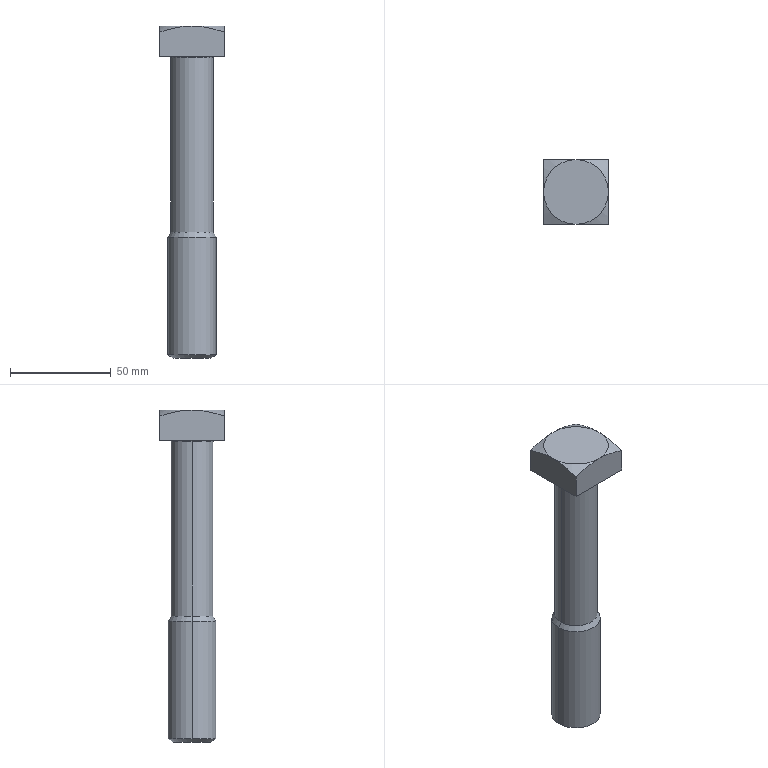Part | SolidWorks | features Cut 1, Extrusion 1, Fillet 1, LPattern 1, RevCut 1, Revolution 1 | 1 solid | 21 faces | box 32.173 x 32.173 x 165 mm | volume 73641 mm3 | cone 8 | plane 7 | cylinder 4 | torus 2 | commonest cylinder face diameters 21 x2 24 x2
STEP:
#1=CARTESIAN_POINT('',(9.402,0.,-150.));
#2=VERTEX_POINT('',#1);
#3=CARTESIAN_POINT('',(-9.402,0.,-150.));
#4=VERTEX_POINT('',#3);
#5=CARTESIAN_POINT('',(0.,0.,-150.));
#6=DIRECTION('',(0.,0.,1.));
#7=DIRECTION('',(1.,0.,0.));
#8=AXIS2_PLACEMENT_3D('',#5,#6,#7);
#9=CIRCLE('',#8,9.402);
#10=EDGE_CURVE('',#2,#4,#9,.T.);
#11=ORIENTED_EDGE('',*,*,#10,.T.);
#12=CARTESIAN_POINT('',(-12.,0.,-148.5));
#13=VERTEX_POINT('',#12);
#14=CARTESIAN_POINT('',(-9.402,0.,-150.));
#15=DIRECTION('',(-0.866,0.,0.5));
#16=VECTOR('',#15,1000.);
#17=LINE('',#14,#16);
#18=EDGE_CURVE('',#4,#13,#17,.T.);
#19=ORIENTED_EDGE('',*,*,#18,.T.);
#20=CARTESIAN_POINT('',(12.,0.,-148.5));
#21=VERTEX_POINT('',#20);
#22=CARTESIAN_POINT('',(0.,0.,-148.5));
#23=DIRECTION('',(0.,0.,1.));
#24=DIRECTION('',(1.,0.,0.));
#25=AXIS2_PLACEMENT_3D('',#22,#23,#24);
#26=CIRCLE('',#25,12.);
#27=EDGE_CURVE('',#21,#13,#26,.T.);
#28=ORIENTED_EDGE('',*,*,#27,.F.);
#29=CARTESIAN_POINT('',(9.402,0.,-150.));
#30=DIRECTION('',(0.866,0.,0.5));
#31=VECTOR('',#30,1000.);
#32=LINE('',#29,#31);
#33=EDGE_CURVE('',#2,#21,#32,.T.);
#34=ORIENTED_EDGE('',*,*,#33,.F.);
#35=EDGE_LOOP('',(#11,#19,#28,#34));
#36=FACE_OUTER_BOUND('',#35,.T.);
#37=CARTESIAN_POINT('',(0.,0.,-150.));
#38=DIRECTION('',(0.,0.,1.));
#39=DIRECTION('',(1.,0.,0.));
#40=AXIS2_PLACEMENT_3D('',#37,#38,#39);
#41=CONICAL_SURFACE('',#40,9.402,1.047);
#42=ADVANCED_FACE('',(#36),#41,.T.);
#43=CARTESIAN_POINT('',(-11.3,0.,0.));
#44=VERTEX_POINT('',#43);
#45=CARTESIAN_POINT('',(11.3,0.,0.));
#46=VERTEX_POINT('',#45);
#47=CARTESIAN_POINT('',(0.,0.,0.));
#48=DIRECTION('',(0.,0.,1.));
#49=DIRECTION('',(1.,0.,0.));
#50=AXIS2_PLACEMENT_3D('',#47,#48,#49);
#51=CIRCLE('',#50,11.3);
#52=EDGE_CURVE('',#44,#46,#51,.T.);
#53=ORIENTED_EDGE('',*,*,#52,.F.);
#54=CARTESIAN_POINT('',(-10.5,0.,-0.8));
#55=VERTEX_POINT('',#54);
#56=CARTESIAN_POINT('',(-11.3,0.,-0.8));
#57=DIRECTION('',(0.,1.,0.));
#58=DIRECTION('',(-1.,0.,0.));
#59=AXIS2_PLACEMENT_3D('',#56,#57,#58);
#60=CIRCLE('',#59,0.8);
#61=EDGE_CURVE('',#44,#55,#60,.T.);
#62=ORIENTED_EDGE('',*,*,#61,.T.);
#63=CARTESIAN_POINT('',(10.5,0.,-0.8));
#64=VERTEX_POINT('',#63);
#65=CARTESIAN_POINT('',(0.,0.,-0.8));
#66=DIRECTION('',(0.,0.,-1.));
#67=DIRECTION('',(1.,0.,0.));
#68=AXIS2_PLACEMENT_3D('',#65,#66,#67);
#69=CIRCLE('',#68,10.5);
#70=EDGE_CURVE('',#64,#55,#69,.T.);
#71=ORIENTED_EDGE('',*,*,#70,.F.);
#72=CARTESIAN_POINT('',(11.3,0.,-0.8));
#73=DIRECTION('',(0.,-1.,0.));
#74=DIRECTION('',(0.,0.,-1.));
#75=AXIS2_PLACEMENT_3D('',#72,#73,#74);
#76=CIRCLE('',#75,0.8);
#77=EDGE_CURVE('',#46,#64,#76,.T.);
#78=ORIENTED_EDGE('',*,*,#77,.F.);
#79=EDGE_LOOP('',(#53,#62,#71,#78));
#80=FACE_OUTER_BOUND('',#79,.T.);
#81=CARTESIAN_POINT('',(0.,0.,-0.8));
#82=DIRECTION('',(0.,0.,1.));
#83=DIRECTION('',(1.,0.,0.));
#84=AXIS2_PLACEMENT_3D('',#81,#82,#83);
#85=TOROIDAL_SURFACE('',#84,11.3,0.8);
#86=ADVANCED_FACE('',(#80),#85,.F.);
#87=CARTESIAN_POINT('',(-12.,0.,-90.));
#88=VERTEX_POINT('',#87);
#89=CARTESIAN_POINT('',(12.,0.,-90.));
#90=VERTEX_POINT('',#89);
#91=CARTESIAN_POINT('',(0.,0.,-90.));
#92=DIRECTION('',(0.,0.,-1.));
#93=DIRECTION('',(-1.,0.,0.));
#94=AXIS2_PLACEMENT_3D('',#91,#92,#93);
#95=CIRCLE('',#94,12.);
#96=EDGE_CURVE('',#88,#90,#95,.T.);
#97=ORIENTED_EDGE('',*,*,#96,.T.);
#98=CARTESIAN_POINT('',(12.,0.,-150.));
#99=DIRECTION('',(0.,0.,-1.));
#100=VECTOR('',#99,1000.);
#101=LINE('',#98,#100);
#102=EDGE_CURVE('',#90,#21,#101,.T.);
#103=ORIENTED_EDGE('',*,*,#102,.T.);
#104=ORIENTED_EDGE('',*,*,#27,.T.);
#105=CARTESIAN_POINT('',(-12.,0.,-150.));
#106=DIRECTION('',(0.,0.,-1.));
#107=VECTOR('',#106,1000.);
#108=LINE('',#105,#107);
#109=EDGE_CURVE('',#88,#13,#108,.T.);
#110=ORIENTED_EDGE('',*,*,#109,.F.);
#111=EDGE_LOOP('',(#97,#103,#104,#110));
#112=FACE_OUTER_BOUND('',#111,.T.);
#113=CARTESIAN_POINT('',(0.,0.,-150.));
#114=DIRECTION('',(0.,0.,-1.));
#115=DIRECTION('',(-1.,0.,0.));
#116=AXIS2_PLACEMENT_3D('',#113,#114,#115);
#117=CYLINDRICAL_SURFACE('',#116,12.);
#118=ADVANCED_FACE('',(#112),#117,.T.);
#119=CARTESIAN_POINT('',(-10.5,0.,-87.402));
#120=VERTEX_POINT('',#119);
#121=CARTESIAN_POINT('',(10.5,0.,-87.402));
#122=VERTEX_POINT('',#121);
#123=CARTESIAN_POINT('',(0.,0.,-87.402));
#124=DIRECTION('',(0.,0.,-1.));
#125=DIRECTION('',(-1.,0.,0.));
#126=AXIS2_PLACEMENT_3D('',#123,#124,#125);
#127=CIRCLE('',#126,10.5);
#128=EDGE_CURVE('',#120,#122,#127,.T.);
#129=ORIENTED_EDGE('',*,*,#128,.T.);
#130=CARTESIAN_POINT('',(10.5,0.,-87.402));
#131=DIRECTION('',(0.5,0.,-0.866));
#132=VECTOR('',#131,1000.);
#133=LINE('',#130,#132);
#134=EDGE_CURVE('',#122,#90,#133,.T.);
#135=ORIENTED_EDGE('',*,*,#134,.T.);
#136=ORIENTED_EDGE('',*,*,#96,.F.);
#137=CARTESIAN_POINT('',(-10.5,0.,-87.402));
#138=DIRECTION('',(-0.5,0.,-0.866));
#139=VECTOR('',#138,1000.);
#140=LINE('',#137,#139);
#141=EDGE_CURVE('',#120,#88,#140,.T.);
#142=ORIENTED_EDGE('',*,*,#141,.F.);
#143=EDGE_LOOP('',(#129,#135,#136,#142));
#144=FACE_OUTER_BOUND('',#143,.T.);
#145=CARTESIAN_POINT('',(0.,0.,-87.402));
#146=DIRECTION('',(0.,0.,-1.));
#147=DIRECTION('',(-1.,0.,0.));
#148=AXIS2_PLACEMENT_3D('',#145,#146,#147);
#149=CONICAL_SURFACE('',#148,10.5,0.5236);
#150=ADVANCED_FACE('',(#144),#149,.T.);
#151=CARTESIAN_POINT('',(0.,0.,-0.8));
#152=DIRECTION('',(0.,0.,-1.));
#153=DIRECTION('',(1.,0.,0.));
#154=AXIS2_PLACEMENT_3D('',#151,#152,#153);
#155=CIRCLE('',#154,10.5);
#156=EDGE_CURVE('',#55,#64,#155,.T.);
#157=ORIENTED_EDGE('',*,*,#156,.T.);
#158=CARTESIAN_POINT('',(10.5,0.,-150.));
#159=DIRECTION('',(0.,0.,-1.));
#160=VECTOR('',#159,1000.);
#161=LINE('',#158,#160);
#162=EDGE_CURVE('',#64,#122,#161,.T.);
#163=ORIENTED_EDGE('',*,*,#162,.T.);
#164=ORIENTED_EDGE('',*,*,#128,.F.);
#165=CARTESIAN_POINT('',(-10.5,0.,-150.));
#166=DIRECTION('',(0.,0.,-1.));
#167=VECTOR('',#166,1000.);
#168=LINE('',#165,#167);
#169=EDGE_CURVE('',#55,#120,#168,.T.);
#170=ORIENTED_EDGE('',*,*,#169,.F.);
#171=EDGE_LOOP('',(#157,#163,#164,#170));
#172=FACE_OUTER_BOUND('',#171,.T.);
#173=CARTESIAN_POINT('',(0.,0.,-150.));
#174=DIRECTION('',(0.,0.,-1.));
#175=DIRECTION('',(-1.,0.,0.));
#176=AXIS2_PLACEMENT_3D('',#173,#174,#175);
#177=CYLINDRICAL_SURFACE('',#176,10.5);
#178=ADVANCED_FACE('',(#172),#177,.T.);
#179=CARTESIAN_POINT('',(0.,0.,0.));
#180=DIRECTION('',(0.,0.,1.));
#181=DIRECTION('',(1.,0.,0.));
#182=AXIS2_PLACEMENT_3D('',#179,#180,#181);
#183=CIRCLE('',#182,11.3);
#184=EDGE_CURVE('',#46,#44,#183,.T.);
#185=ORIENTED_EDGE('',*,*,#184,.T.);
#186=ORIENTED_EDGE('',*,*,#52,.T.);
#187=EDGE_LOOP('',(#185,#186));
#188=FACE_BOUND('',#187,.T.);
#189=CARTESIAN_POINT('',(-16.087,16.087,0.));
#190=VERTEX_POINT('',#189);
#191=CARTESIAN_POINT('',(-16.087,-16.087,0.));
#192=VERTEX_POINT('',#191);
#193=CARTESIAN_POINT('',(-16.087,16.087,0.));
#194=DIRECTION('',(0.,-1.,0.));
#195=VECTOR('',#194,1000.);
#196=LINE('',#193,#195);
#197=EDGE_CURVE('',#190,#192,#196,.T.);
#198=ORIENTED_EDGE('',*,*,#197,.F.);
#199=CARTESIAN_POINT('',(16.087,16.087,0.));
#200=VERTEX_POINT('',#199);
#201=CARTESIAN_POINT('',(-16.087,16.087,0.));
#202=DIRECTION('',(-1.,0.,0.));
#203=VECTOR('',#202,1000.);
#204=LINE('',#201,#203);
#205=EDGE_CURVE('',#200,#190,#204,.T.);
#206=ORIENTED_EDGE('',*,*,#205,.F.);
#207=CARTESIAN_POINT('',(16.087,-16.087,0.));
#208=VERTEX_POINT('',#207);
#209=CARTESIAN_POINT('',(16.087,16.087,0.));
#210=DIRECTION('',(0.,1.,0.));
#211=VECTOR('',#210,1000.);
#212=LINE('',#209,#211);
#213=EDGE_CURVE('',#208,#200,#212,.T.);
#214=ORIENTED_EDGE('',*,*,#213,.F.);
#215=CARTESIAN_POINT('',(-16.087,-16.087,0.));
#216=DIRECTION('',(1.,0.,0.));
#217=VECTOR('',#216,1000.);
#218=LINE('',#215,#217);
#219=EDGE_CURVE('',#192,#208,#218,.T.);
#220=ORIENTED_EDGE('',*,*,#219,.F.);
#221=EDGE_LOOP('',(#198,#206,#214,#220));
#222=FACE_OUTER_BOUND('',#221,.T.);
#223=CARTESIAN_POINT('',(-16.087,-16.087,0.));
#224=DIRECTION('',(0.,0.,1.));
#225=DIRECTION('',(1.,0.,0.));
#226=AXIS2_PLACEMENT_3D('',#223,#224,#225);
#227=PLANE('',#226);
#228=ADVANCED_FACE('',(#188,#222),#227,.F.);
#229=CARTESIAN_POINT('',(-16.087,16.087,11.893));
#230=VERTEX_POINT('',#229);
#231=CARTESIAN_POINT('',(-16.087,0.,15.));
#232=VERTEX_POINT('',#231);
#233=CARTESIAN_POINT('',(-16.087,16.087,11.893));
#234=CARTESIAN_POINT('',(-16.087,14.791,12.32));
#235=CARTESIAN_POINT('',(-16.087,13.489,12.724));
#236=CARTESIAN_POINT('',(-16.087,10.862,13.463));
#237=CARTESIAN_POINT('',(-16.087,9.539,13.798));
#238=CARTESIAN_POINT('',(-16.087,6.86,14.365));
#239=CARTESIAN_POINT('',(-16.087,5.504,14.597));
#240=CARTESIAN_POINT('',(-16.087,3.438,14.837));
#241=CARTESIAN_POINT('',(-16.087,2.745,14.898));
#242=CARTESIAN_POINT('',(-16.087,1.369,14.98));
#243=CARTESIAN_POINT('',(-16.087,0.6835,15.));
#244=CARTESIAN_POINT('',(-16.087,0.,15.));
#245=B_SPLINE_CURVE_WITH_KNOTS('',3,(#233,#234,#235,#236,#237,#238,#239,#240,#241,#242,#243,#244),.UNSPECIFIED.,.F.,.F.,(4,2,2,2,2,4),(0.01378,0.01787,0.02196,0.02605,0.0281,0.03014),.UNSPECIFIED.);
#246=EDGE_CURVE('',#230,#232,#245,.T.);
#247=ORIENTED_EDGE('',*,*,#246,.F.);
#248=CARTESIAN_POINT('',(-16.087,16.087,15.));
#249=DIRECTION('',(0.,0.,-1.));
#250=VECTOR('',#249,1000.);
#251=LINE('',#248,#250);
#252=EDGE_CURVE('',#230,#190,#251,.T.);
#253=ORIENTED_EDGE('',*,*,#252,.T.);
#254=ORIENTED_EDGE('',*,*,#197,.T.);
#255=CARTESIAN_POINT('',(-16.087,-16.087,11.893));
#256=VERTEX_POINT('',#255);
#257=CARTESIAN_POINT('',(-16.087,-16.087,15.));
#258=DIRECTION('',(0.,0.,-1.));
#259=VECTOR('',#258,1000.);
#260=LINE('',#257,#259);
#261=EDGE_CURVE('',#256,#192,#260,.T.);
#262=ORIENTED_EDGE('',*,*,#261,.F.);
#263=CARTESIAN_POINT('',(-16.087,0.,15.));
#264=CARTESIAN_POINT('',(-16.087,-1.371,15.));
#265=CARTESIAN_POINT('',(-16.087,-2.733,14.917));
#266=CARTESIAN_POINT('',(-16.087,-5.441,14.606));
#267=CARTESIAN_POINT('',(-16.087,-6.786,14.379));
#268=CARTESIAN_POINT('',(-16.087,-9.466,13.816));
#269=CARTESIAN_POINT('',(-16.087,-10.799,13.48));
#270=CARTESIAN_POINT('',(-16.087,-13.458,12.734));
#271=CARTESIAN_POINT('',(-16.087,-14.777,12.325));
#272=CARTESIAN_POINT('',(-16.087,-16.087,11.893));
#273=B_SPLINE_CURVE_WITH_KNOTS('',3,(#263,#264,#265,#266,#267,#268,#269,#270,#271,#272),.UNSPECIFIED.,.F.,.F.,(4,2,2,2,4),(0.03014,0.03425,0.03835,0.04246,0.04656),.UNSPECIFIED.);
#274=EDGE_CURVE('',#232,#256,#273,.T.);
#275=ORIENTED_EDGE('',*,*,#274,.F.);
#276=EDGE_LOOP('',(#247,#253,#254,#262,#275));
#277=FACE_OUTER_BOUND('',#276,.T.);
#278=CARTESIAN_POINT('',(-16.087,16.087,15.));
#279=DIRECTION('',(1.,0.,0.));
#280=DIRECTION('',(0.,1.,0.));
#281=AXIS2_PLACEMENT_3D('',#278,#279,#280);
#282=PLANE('',#281);
#283=ADVANCED_FACE('',(#277),#282,.F.);
#284=CARTESIAN_POINT('',(0.,-16.087,15.));
#285=VERTEX_POINT('',#284);
#286=CARTESIAN_POINT('',(-16.087,-16.087,11.893));
#287=CARTESIAN_POINT('',(-14.777,-16.087,12.325));
#288=CARTESIAN_POINT('',(-13.458,-16.087,12.734));
#289=CARTESIAN_POINT('',(-10.799,-16.087,13.48));
#290=CARTESIAN_POINT('',(-9.466,-16.087,13.816));
#291=CARTESIAN_POINT('',(-6.786,-16.087,14.379));
#292=CARTESIAN_POINT('',(-5.441,-16.087,14.606));
#293=CARTESIAN_POINT('',(-2.733,-16.087,14.917));
#294=CARTESIAN_POINT('',(-1.371,-16.087,15.));
#295=CARTESIAN_POINT('',(0.,-16.087,15.));
#296=B_SPLINE_CURVE_WITH_KNOTS('',3,(#286,#287,#288,#289,#290,#291,#292,#293,#294,#295),.UNSPECIFIED.,.F.,.F.,(4,2,2,2,4),(0.01765,0.02179,0.02592,0.03005,0.03419),.UNSPECIFIED.);
#297=EDGE_CURVE('',#256,#285,#296,.T.);
#298=ORIENTED_EDGE('',*,*,#297,.F.);
#299=ORIENTED_EDGE('',*,*,#261,.T.);
#300=ORIENTED_EDGE('',*,*,#219,.T.);
#301=CARTESIAN_POINT('',(16.087,-16.087,11.893));
#302=VERTEX_POINT('',#301);
#303=CARTESIAN_POINT('',(16.087,-16.087,15.));
#304=DIRECTION('',(0.,0.,-1.));
#305=VECTOR('',#304,1000.);
#306=LINE('',#303,#305);
#307=EDGE_CURVE('',#302,#208,#306,.T.);
#308=ORIENTED_EDGE('',*,*,#307,.F.);
#309=CARTESIAN_POINT('',(0.,-16.087,15.));
#310=CARTESIAN_POINT('',(0.6835,-16.087,15.));
#311=CARTESIAN_POINT('',(1.369,-16.087,14.98));
#312=CARTESIAN_POINT('',(2.745,-16.087,14.898));
#313=CARTESIAN_POINT('',(3.438,-16.087,14.837));
#314=CARTESIAN_POINT('',(5.504,-16.087,14.597));
#315=CARTESIAN_POINT('',(6.86,-16.087,14.365));
#316=CARTESIAN_POINT('',(9.539,-16.087,13.798));
#317=CARTESIAN_POINT('',(10.862,-16.087,13.463));
#318=CARTESIAN_POINT('',(13.489,-16.087,12.724));
#319=CARTESIAN_POINT('',(14.791,-16.087,12.32));
#320=CARTESIAN_POINT('',(16.087,-16.087,11.893));
#321=B_SPLINE_CURVE_WITH_KNOTS('',3,(#309,#310,#311,#312,#313,#314,#315,#316,#317,#318,#319,#320),.UNSPECIFIED.,.F.,.F.,(4,2,2,2,2,4),(0.03419,0.03625,0.03831,0.04243,0.04655,0.05067),.UNSPECIFIED.);
#322=EDGE_CURVE('',#285,#302,#321,.T.);
#323=ORIENTED_EDGE('',*,*,#322,.F.);
#324=EDGE_LOOP('',(#298,#299,#300,#308,#323));
#325=FACE_OUTER_BOUND('',#324,.T.);
#326=CARTESIAN_POINT('',(-16.087,-16.087,15.));
#327=DIRECTION('',(0.,1.,0.));
#328=DIRECTION('',(0.,0.,1.));
#329=AXIS2_PLACEMENT_3D('',#326,#327,#328);
#330=PLANE('',#329);
#331=ADVANCED_FACE('',(#325),#330,.F.);
#332=CARTESIAN_POINT('',(16.087,0.,15.));
#333=VERTEX_POINT('',#332);
#334=CARTESIAN_POINT('',(16.087,-16.087,11.893));
#335=CARTESIAN_POINT('',(16.087,-14.777,12.325));
#336=CARTESIAN_POINT('',(16.087,-13.458,12.734));
#337=CARTESIAN_POINT('',(16.087,-10.799,13.48));
#338=CARTESIAN_POINT('',(16.087,-9.466,13.816));
#339=CARTESIAN_POINT('',(16.087,-6.786,14.379));
#340=CARTESIAN_POINT('',(16.087,-5.441,14.606));
#341=CARTESIAN_POINT('',(16.087,-2.733,14.917));
#342=CARTESIAN_POINT('',(16.087,-1.371,15.));
#343=CARTESIAN_POINT('',(16.087,0.,15.));
#344=B_SPLINE_CURVE_WITH_KNOTS('',3,(#334,#335,#336,#337,#338,#339,#340,#341,#342,#343),.UNSPECIFIED.,.F.,.F.,(4,2,2,2,4),(0.01765,0.02179,0.02592,0.03005,0.03419),.UNSPECIFIED.);
#345=EDGE_CURVE('',#302,#333,#344,.T.);
#346=ORIENTED_EDGE('',*,*,#345,.F.);
#347=ORIENTED_EDGE('',*,*,#307,.T.);
#348=ORIENTED_EDGE('',*,*,#213,.T.);
#349=CARTESIAN_POINT('',(16.087,16.087,11.893));
#350=VERTEX_POINT('',#349);
#351=CARTESIAN_POINT('',(16.087,16.087,15.));
#352=DIRECTION('',(0.,0.,-1.));
#353=VECTOR('',#352,1000.);
#354=LINE('',#351,#353);
#355=EDGE_CURVE('',#350,#200,#354,.T.);
#356=ORIENTED_EDGE('',*,*,#355,.F.);
#357=CARTESIAN_POINT('',(16.087,0.,15.));
#358=CARTESIAN_POINT('',(16.087,0.6835,15.));
#359=CARTESIAN_POINT('',(16.087,1.369,14.98));
#360=CARTESIAN_POINT('',(16.087,2.745,14.898));
#361=CARTESIAN_POINT('',(16.087,3.438,14.837));
#362=CARTESIAN_POINT('',(16.087,5.504,14.597));
#363=CARTESIAN_POINT('',(16.087,6.86,14.365));
#364=CARTESIAN_POINT('',(16.087,9.539,13.798));
#365=CARTESIAN_POINT('',(16.087,10.862,13.463));
#366=CARTESIAN_POINT('',(16.087,13.489,12.724));
#367=CARTESIAN_POINT('',(16.087,14.791,12.32));
#368=CARTESIAN_POINT('',(16.087,16.087,11.893));
#369=B_SPLINE_CURVE_WITH_KNOTS('',3,(#357,#358,#359,#360,#361,#362,#363,#364,#365,#366,#367,#368),.UNSPECIFIED.,.F.,.F.,(4,2,2,2,2,4),(0.03419,0.03625,0.03831,0.04243,0.04655,0.05067),.UNSPECIFIED.);
#370=EDGE_CURVE('',#333,#350,#369,.T.);
#371=ORIENTED_EDGE('',*,*,#370,.F.);
#372=EDGE_LOOP('',(#346,#347,#348,#356,#371));
#373=FACE_OUTER_BOUND('',#372,.T.);
#374=CARTESIAN_POINT('',(16.087,16.087,15.));
#375=DIRECTION('',(-1.,0.,0.));
#376=DIRECTION('',(0.,-1.,0.));
#377=AXIS2_PLACEMENT_3D('',#374,#375,#376);
#378=PLANE('',#377);
#379=ADVANCED_FACE('',(#373),#378,.F.);
#380=CARTESIAN_POINT('',(0.,16.087,15.));
#381=VERTEX_POINT('',#380);
#382=CARTESIAN_POINT('',(16.087,16.087,11.893));
#383=CARTESIAN_POINT('',(14.791,16.087,12.32));
#384=CARTESIAN_POINT('',(13.489,16.087,12.724));
#385=CARTESIAN_POINT('',(10.862,16.087,13.463));
#386=CARTESIAN_POINT('',(9.539,16.087,13.798));
#387=CARTESIAN_POINT('',(6.86,16.087,14.365));
#388=CARTESIAN_POINT('',(5.504,16.087,14.597));
#389=CARTESIAN_POINT('',(3.438,16.087,14.837));
#390=CARTESIAN_POINT('',(2.745,16.087,14.898));
#391=CARTESIAN_POINT('',(1.369,16.087,14.98));
#392=CARTESIAN_POINT('',(0.6835,16.087,15.));
#393=CARTESIAN_POINT('',(0.,16.087,15.));
#394=B_SPLINE_CURVE_WITH_KNOTS('',3,(#382,#383,#384,#385,#386,#387,#388,#389,#390,#391,#392,#393),.UNSPECIFIED.,.F.,.F.,(4,2,2,2,2,4),(0.01378,0.01787,0.02196,0.02605,0.0281,0.03014),.UNSPECIFIED.);
#395=EDGE_CURVE('',#350,#381,#394,.T.);
#396=ORIENTED_EDGE('',*,*,#395,.F.);
#397=ORIENTED_EDGE('',*,*,#355,.T.);
#398=ORIENTED_EDGE('',*,*,#205,.T.);
#399=ORIENTED_EDGE('',*,*,#252,.F.);
#400=CARTESIAN_POINT('',(0.,16.087,15.));
#401=CARTESIAN_POINT('',(-1.371,16.087,15.));
#402=CARTESIAN_POINT('',(-2.733,16.087,14.917));
#403=CARTESIAN_POINT('',(-5.441,16.087,14.606));
#404=CARTESIAN_POINT('',(-6.786,16.087,14.379));
#405=CARTESIAN_POINT('',(-9.466,16.087,13.816));
#406=CARTESIAN_POINT('',(-10.799,16.087,13.48));
#407=CARTESIAN_POINT('',(-13.458,16.087,12.734));
#408=CARTESIAN_POINT('',(-14.777,16.087,12.325));
#409=CARTESIAN_POINT('',(-16.087,16.087,11.893));
#410=B_SPLINE_CURVE_WITH_KNOTS('',3,(#400,#401,#402,#403,#404,#405,#406,#407,#408,#409),.UNSPECIFIED.,.F.,.F.,(4,2,2,2,4),(0.03014,0.03425,0.03835,0.04246,0.04656),.UNSPECIFIED.);
#411=EDGE_CURVE('',#381,#230,#410,.T.);
#412=ORIENTED_EDGE('',*,*,#411,.F.);
#413=EDGE_LOOP('',(#396,#397,#398,#399,#412));
#414=FACE_OUTER_BOUND('',#413,.T.);
#415=CARTESIAN_POINT('',(-16.087,16.087,15.));
#416=DIRECTION('',(0.,-1.,0.));
#417=DIRECTION('',(0.,0.,-1.));
#418=AXIS2_PLACEMENT_3D('',#415,#416,#417);
#419=PLANE('',#418);
#420=ADVANCED_FACE('',(#414),#419,.F.);
#421=ORIENTED_EDGE('',*,*,#322,.T.);
#422=ORIENTED_EDGE('',*,*,#345,.T.);
#423=CARTESIAN_POINT('',(0.,0.,15.));
#424=DIRECTION('',(0.,0.,1.));
#425=DIRECTION('',(1.,0.,0.));
#426=AXIS2_PLACEMENT_3D('',#423,#424,#425);
#427=CIRCLE('',#426,16.087);
#428=EDGE_CURVE('',#285,#333,#427,.T.);
#429=ORIENTED_EDGE('',*,*,#428,.F.);
#430=EDGE_LOOP('',(#421,#422,#429));
#431=FACE_OUTER_BOUND('',#430,.T.);
#432=CARTESIAN_POINT('',(0.,0.,15.));
#433=DIRECTION('',(0.,0.,-1.));
#434=DIRECTION('',(1.,0.,0.));
#435=AXIS2_PLACEMENT_3D('',#432,#433,#434);
#436=CONICAL_SURFACE('',#435,16.087,1.134);
#437=ADVANCED_FACE('',(#431),#436,.T.);
#438=ORIENTED_EDGE('',*,*,#274,.T.);
#439=ORIENTED_EDGE('',*,*,#297,.T.);
#440=CARTESIAN_POINT('',(0.,0.,15.));
#441=DIRECTION('',(0.,0.,1.));
#442=DIRECTION('',(1.,0.,0.));
#443=AXIS2_PLACEMENT_3D('',#440,#441,#442);
#444=CIRCLE('',#443,16.087);
#445=EDGE_CURVE('',#232,#285,#444,.T.);
#446=ORIENTED_EDGE('',*,*,#445,.F.);
#447=EDGE_LOOP('',(#438,#439,#446));
#448=FACE_OUTER_BOUND('',#447,.T.);
#449=CARTESIAN_POINT('',(0.,0.,15.));
#450=DIRECTION('',(0.,0.,-1.));
#451=DIRECTION('',(1.,0.,0.));
#452=AXIS2_PLACEMENT_3D('',#449,#450,#451);
#453=CONICAL_SURFACE('',#452,16.087,1.134);
#454=ADVANCED_FACE('',(#448),#453,.T.);
#455=ORIENTED_EDGE('',*,*,#246,.T.);
#456=CARTESIAN_POINT('',(0.,0.,15.));
#457=DIRECTION('',(0.,0.,1.));
#458=DIRECTION('',(1.,0.,0.));
#459=AXIS2_PLACEMENT_3D('',#456,#457,#458);
#460=CIRCLE('',#459,16.087);
#461=EDGE_CURVE('',#381,#232,#460,.T.);
#462=ORIENTED_EDGE('',*,*,#461,.F.);
#463=ORIENTED_EDGE('',*,*,#411,.T.);
#464=EDGE_LOOP('',(#455,#462,#463));
#465=FACE_OUTER_BOUND('',#464,.T.);
#466=CARTESIAN_POINT('',(0.,0.,15.));
#467=DIRECTION('',(0.,0.,-1.));
#468=DIRECTION('',(1.,0.,0.));
#469=AXIS2_PLACEMENT_3D('',#466,#467,#468);
#470=CONICAL_SURFACE('',#469,16.087,1.134);
#471=ADVANCED_FACE('',(#465),#470,.T.);
#472=ORIENTED_EDGE('',*,*,#370,.T.);
#473=ORIENTED_EDGE('',*,*,#395,.T.);
#474=CARTESIAN_POINT('',(0.,0.,15.));
#475=DIRECTION('',(0.,0.,1.));
#476=DIRECTION('',(1.,0.,0.));
#477=AXIS2_PLACEMENT_3D('',#474,#475,#476);
#478=CIRCLE('',#477,16.087);
#479=EDGE_CURVE('',#333,#381,#478,.T.);
#480=ORIENTED_EDGE('',*,*,#479,.F.);
#481=EDGE_LOOP('',(#472,#473,#480));
#482=FACE_OUTER_BOUND('',#481,.T.);
#483=CARTESIAN_POINT('',(0.,0.,15.));
#484=DIRECTION('',(0.,0.,-1.));
#485=DIRECTION('',(1.,0.,0.));
#486=AXIS2_PLACEMENT_3D('',#483,#484,#485);
#487=CONICAL_SURFACE('',#486,16.087,1.134);
#488=ADVANCED_FACE('',(#482),#487,.T.);
#489=ORIENTED_EDGE('',*,*,#428,.T.);
#490=ORIENTED_EDGE('',*,*,#479,.T.);
#491=ORIENTED_EDGE('',*,*,#461,.T.);
#492=ORIENTED_EDGE('',*,*,#445,.T.);
#493=EDGE_LOOP('',(#489,#490,#491,#492));
#494=FACE_OUTER_BOUND('',#493,.T.);
#495=CARTESIAN_POINT('',(-16.087,-16.087,15.));
#496=DIRECTION('',(0.,0.,1.));
#497=DIRECTION('',(1.,0.,0.));
#498=AXIS2_PLACEMENT_3D('',#495,#496,#497);
#499=PLANE('',#498);
#500=ADVANCED_FACE('',(#494),#499,.T.);
#501=ORIENTED_EDGE('',*,*,#162,.F.);
#502=ORIENTED_EDGE('',*,*,#70,.T.);
#503=ORIENTED_EDGE('',*,*,#169,.T.);
#504=CARTESIAN_POINT('',(0.,0.,-87.402));
#505=DIRECTION('',(0.,0.,-1.));
#506=DIRECTION('',(-1.,0.,0.));
#507=AXIS2_PLACEMENT_3D('',#504,#505,#506);
#508=CIRCLE('',#507,10.5);
#509=EDGE_CURVE('',#122,#120,#508,.T.);
#510=ORIENTED_EDGE('',*,*,#509,.F.);
#511=EDGE_LOOP('',(#501,#502,#503,#510));
#512=FACE_OUTER_BOUND('',#511,.T.);
#513=CARTESIAN_POINT('',(0.,0.,-150.));
#514=DIRECTION('',(0.,0.,-1.));
#515=DIRECTION('',(-1.,0.,0.));
#516=AXIS2_PLACEMENT_3D('',#513,#514,#515);
#517=CYLINDRICAL_SURFACE('',#516,10.5);
#518=ADVANCED_FACE('',(#512),#517,.T.);
#519=ORIENTED_EDGE('',*,*,#134,.F.);
#520=ORIENTED_EDGE('',*,*,#509,.T.);
#521=ORIENTED_EDGE('',*,*,#141,.T.);
#522=CARTESIAN_POINT('',(0.,0.,-90.));
#523=DIRECTION('',(0.,0.,-1.));
#524=DIRECTION('',(-1.,0.,0.));
#525=AXIS2_PLACEMENT_3D('',#522,#523,#524);
#526=CIRCLE('',#525,12.);
#527=EDGE_CURVE('',#90,#88,#526,.T.);
#528=ORIENTED_EDGE('',*,*,#527,.F.);
#529=EDGE_LOOP('',(#519,#520,#521,#528));
#530=FACE_OUTER_BOUND('',#529,.T.);
#531=CARTESIAN_POINT('',(0.,0.,-87.402));
#532=DIRECTION('',(0.,0.,-1.));
#533=DIRECTION('',(-1.,0.,0.));
#534=AXIS2_PLACEMENT_3D('',#531,#532,#533);
#535=CONICAL_SURFACE('',#534,10.5,0.5236);
#536=ADVANCED_FACE('',(#530),#535,.T.);
#537=ORIENTED_EDGE('',*,*,#102,.F.);
#538=ORIENTED_EDGE('',*,*,#527,.T.);
#539=ORIENTED_EDGE('',*,*,#109,.T.);
#540=CARTESIAN_POINT('',(0.,0.,-148.5));
#541=DIRECTION('',(0.,0.,1.));
#542=DIRECTION('',(1.,0.,0.));
#543=AXIS2_PLACEMENT_3D('',#540,#541,#542);
#544=CIRCLE('',#543,12.);
#545=EDGE_CURVE('',#13,#21,#544,.T.);
#546=ORIENTED_EDGE('',*,*,#545,.T.);
#547=EDGE_LOOP('',(#537,#538,#539,#546));
#548=FACE_OUTER_BOUND('',#547,.T.);
#549=CARTESIAN_POINT('',(0.,0.,-150.));
#550=DIRECTION('',(0.,0.,-1.));
#551=DIRECTION('',(-1.,0.,0.));
#552=AXIS2_PLACEMENT_3D('',#549,#550,#551);
#553=CYLINDRICAL_SURFACE('',#552,12.);
#554=ADVANCED_FACE('',(#548),#553,.T.);
#555=ORIENTED_EDGE('',*,*,#61,.F.);
#556=ORIENTED_EDGE('',*,*,#184,.F.);
#557=ORIENTED_EDGE('',*,*,#77,.T.);
#558=ORIENTED_EDGE('',*,*,#156,.F.);
#559=EDGE_LOOP('',(#555,#556,#557,#558));
#560=FACE_OUTER_BOUND('',#559,.T.);
#561=CARTESIAN_POINT('',(0.,0.,-0.8));
#562=DIRECTION('',(0.,0.,1.));
#563=DIRECTION('',(1.,0.,0.));
#564=AXIS2_PLACEMENT_3D('',#561,#562,#563);
#565=TOROIDAL_SURFACE('',#564,11.3,0.8);
#566=ADVANCED_FACE('',(#560),#565,.F.);
#567=ORIENTED_EDGE('',*,*,#18,.F.);
#568=CARTESIAN_POINT('',(0.,0.,-150.));
#569=DIRECTION('',(0.,0.,1.));
#570=DIRECTION('',(1.,0.,0.));
#571=AXIS2_PLACEMENT_3D('',#568,#569,#570);
#572=CIRCLE('',#571,9.402);
#573=EDGE_CURVE('',#4,#2,#572,.T.);
#574=ORIENTED_EDGE('',*,*,#573,.T.);
#575=ORIENTED_EDGE('',*,*,#33,.T.);
#576=ORIENTED_EDGE('',*,*,#545,.F.);
#577=EDGE_LOOP('',(#567,#574,#575,#576));
#578=FACE_OUTER_BOUND('',#577,.T.);
#579=CARTESIAN_POINT('',(0.,0.,-150.));
#580=DIRECTION('',(0.,0.,1.));
#581=DIRECTION('',(1.,0.,0.));
#582=AXIS2_PLACEMENT_3D('',#579,#580,#581);
#583=CONICAL_SURFACE('',#582,9.402,1.047);
#584=ADVANCED_FACE('',(#578),#583,.T.);
#585=ORIENTED_EDGE('',*,*,#10,.F.);
#586=ORIENTED_EDGE('',*,*,#573,.F.);
#587=EDGE_LOOP('',(#585,#586));
#588=FACE_OUTER_BOUND('',#587,.T.);
#589=CARTESIAN_POINT('',(12.,0.,-150.));
#590=DIRECTION('',(0.,0.,1.));
#591=DIRECTION('',(1.,0.,0.));
#592=AXIS2_PLACEMENT_3D('',#589,#590,#591);
#593=PLANE('',#592);
#594=ADVANCED_FACE('',(#588),#593,.F.);
#595=CLOSED_SHELL('',(#42,#86,#118,#150,#178,#228,#283,#331,#379,#420,#437,#454,#471,#488,#500,#518,#536,#554,#566,#584,#594));
#596=MANIFOLD_SOLID_BREP('',#595);
#597=CARTESIAN_POINT('',(0.,0.,0.));
#598=DIRECTION('',(0.,0.,1.));
#599=DIRECTION('',(1.,0.,0.));
#600=AXIS2_PLACEMENT_3D('',#597,#598,#599);
#601=(LENGTH_UNIT()NAMED_UNIT(*)SI_UNIT(.MILLI.,.METRE.));
#602=UNCERTAINTY_MEASURE_WITH_UNIT(LENGTH_MEASURE(0.00001),#601,'','');
#603=(NAMED_UNIT(*)PLANE_ANGLE_UNIT()SI_UNIT($,.RADIAN.));
#604=(NAMED_UNIT(*)SI_UNIT($,.STERADIAN.)SOLID_ANGLE_UNIT());
#605=(GEOMETRIC_REPRESENTATION_CONTEXT(3)GLOBAL_UNCERTAINTY_ASSIGNED_CONTEXT((#602))GLOBAL_UNIT_ASSIGNED_CONTEXT((#601,#603,#604))REPRESENTATION_CONTEXT('',''));
#606=ADVANCED_BREP_SHAPE_REPRESENTATION('',(#596,#600),#605);